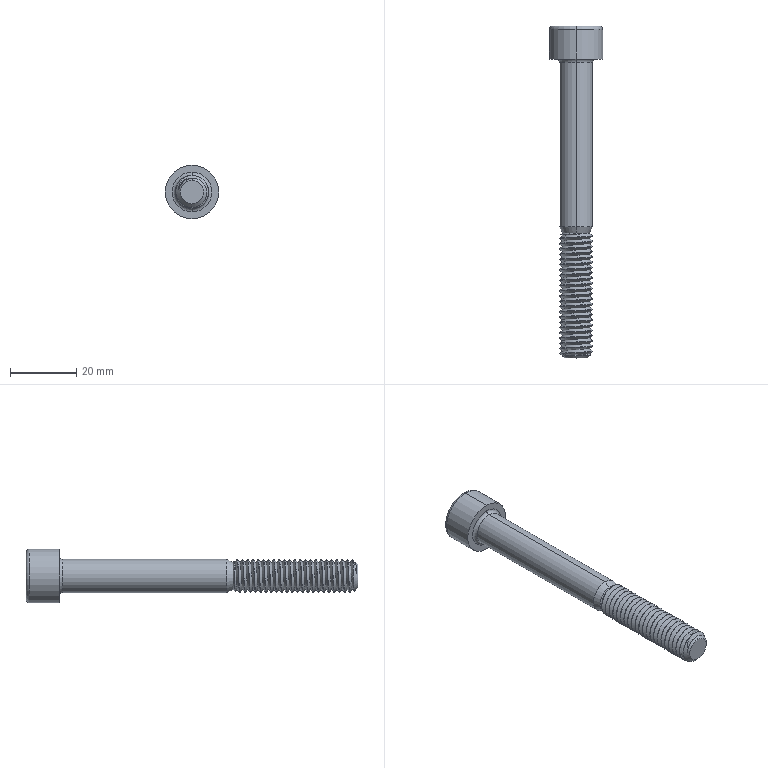Part | STEP file | Parafuso M10 - 90mm | 1 solid | 77 faces | box 16.1 x 100 x 16.1 mm | volume 8134 mm3 | cylinder 50 | plane 10 | cone 9 | torus 6 | spline 2 | commonest cylinder face diameters 10 x48 16.1 x2